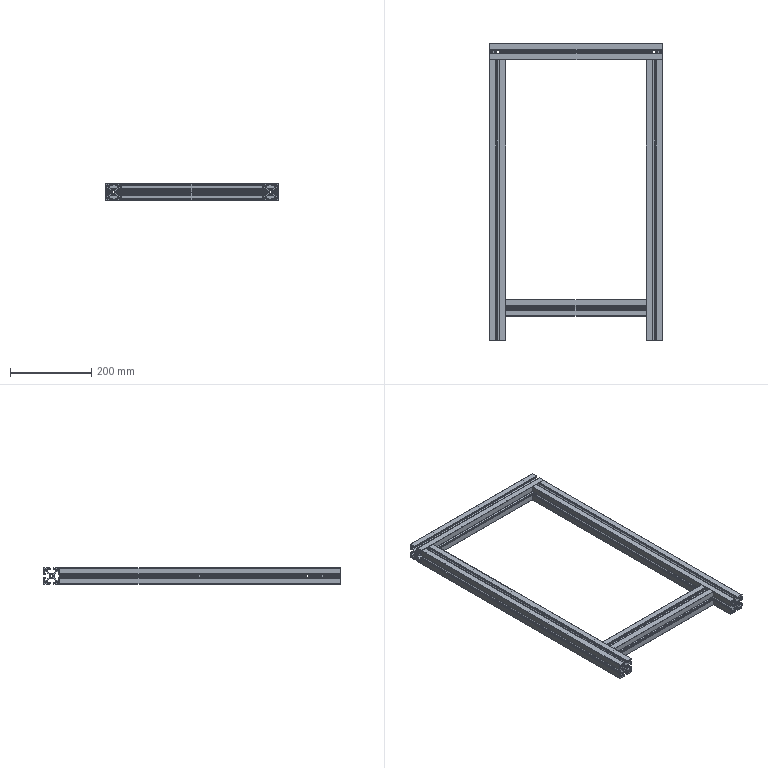Part | SolidWorks | features ICE 3, WeldMemberFeat 1, WeldmentFeature 1 | 4 solids | 848 faces | box 425 x 730.5 x 40 mm | volume 1437708 mm3 | cylinder 467 | plane 381 | commonest cylinder face diameters 1 x184 0.6 x155 4 x52 4.9 x32 6.8 x16 8.8 x10